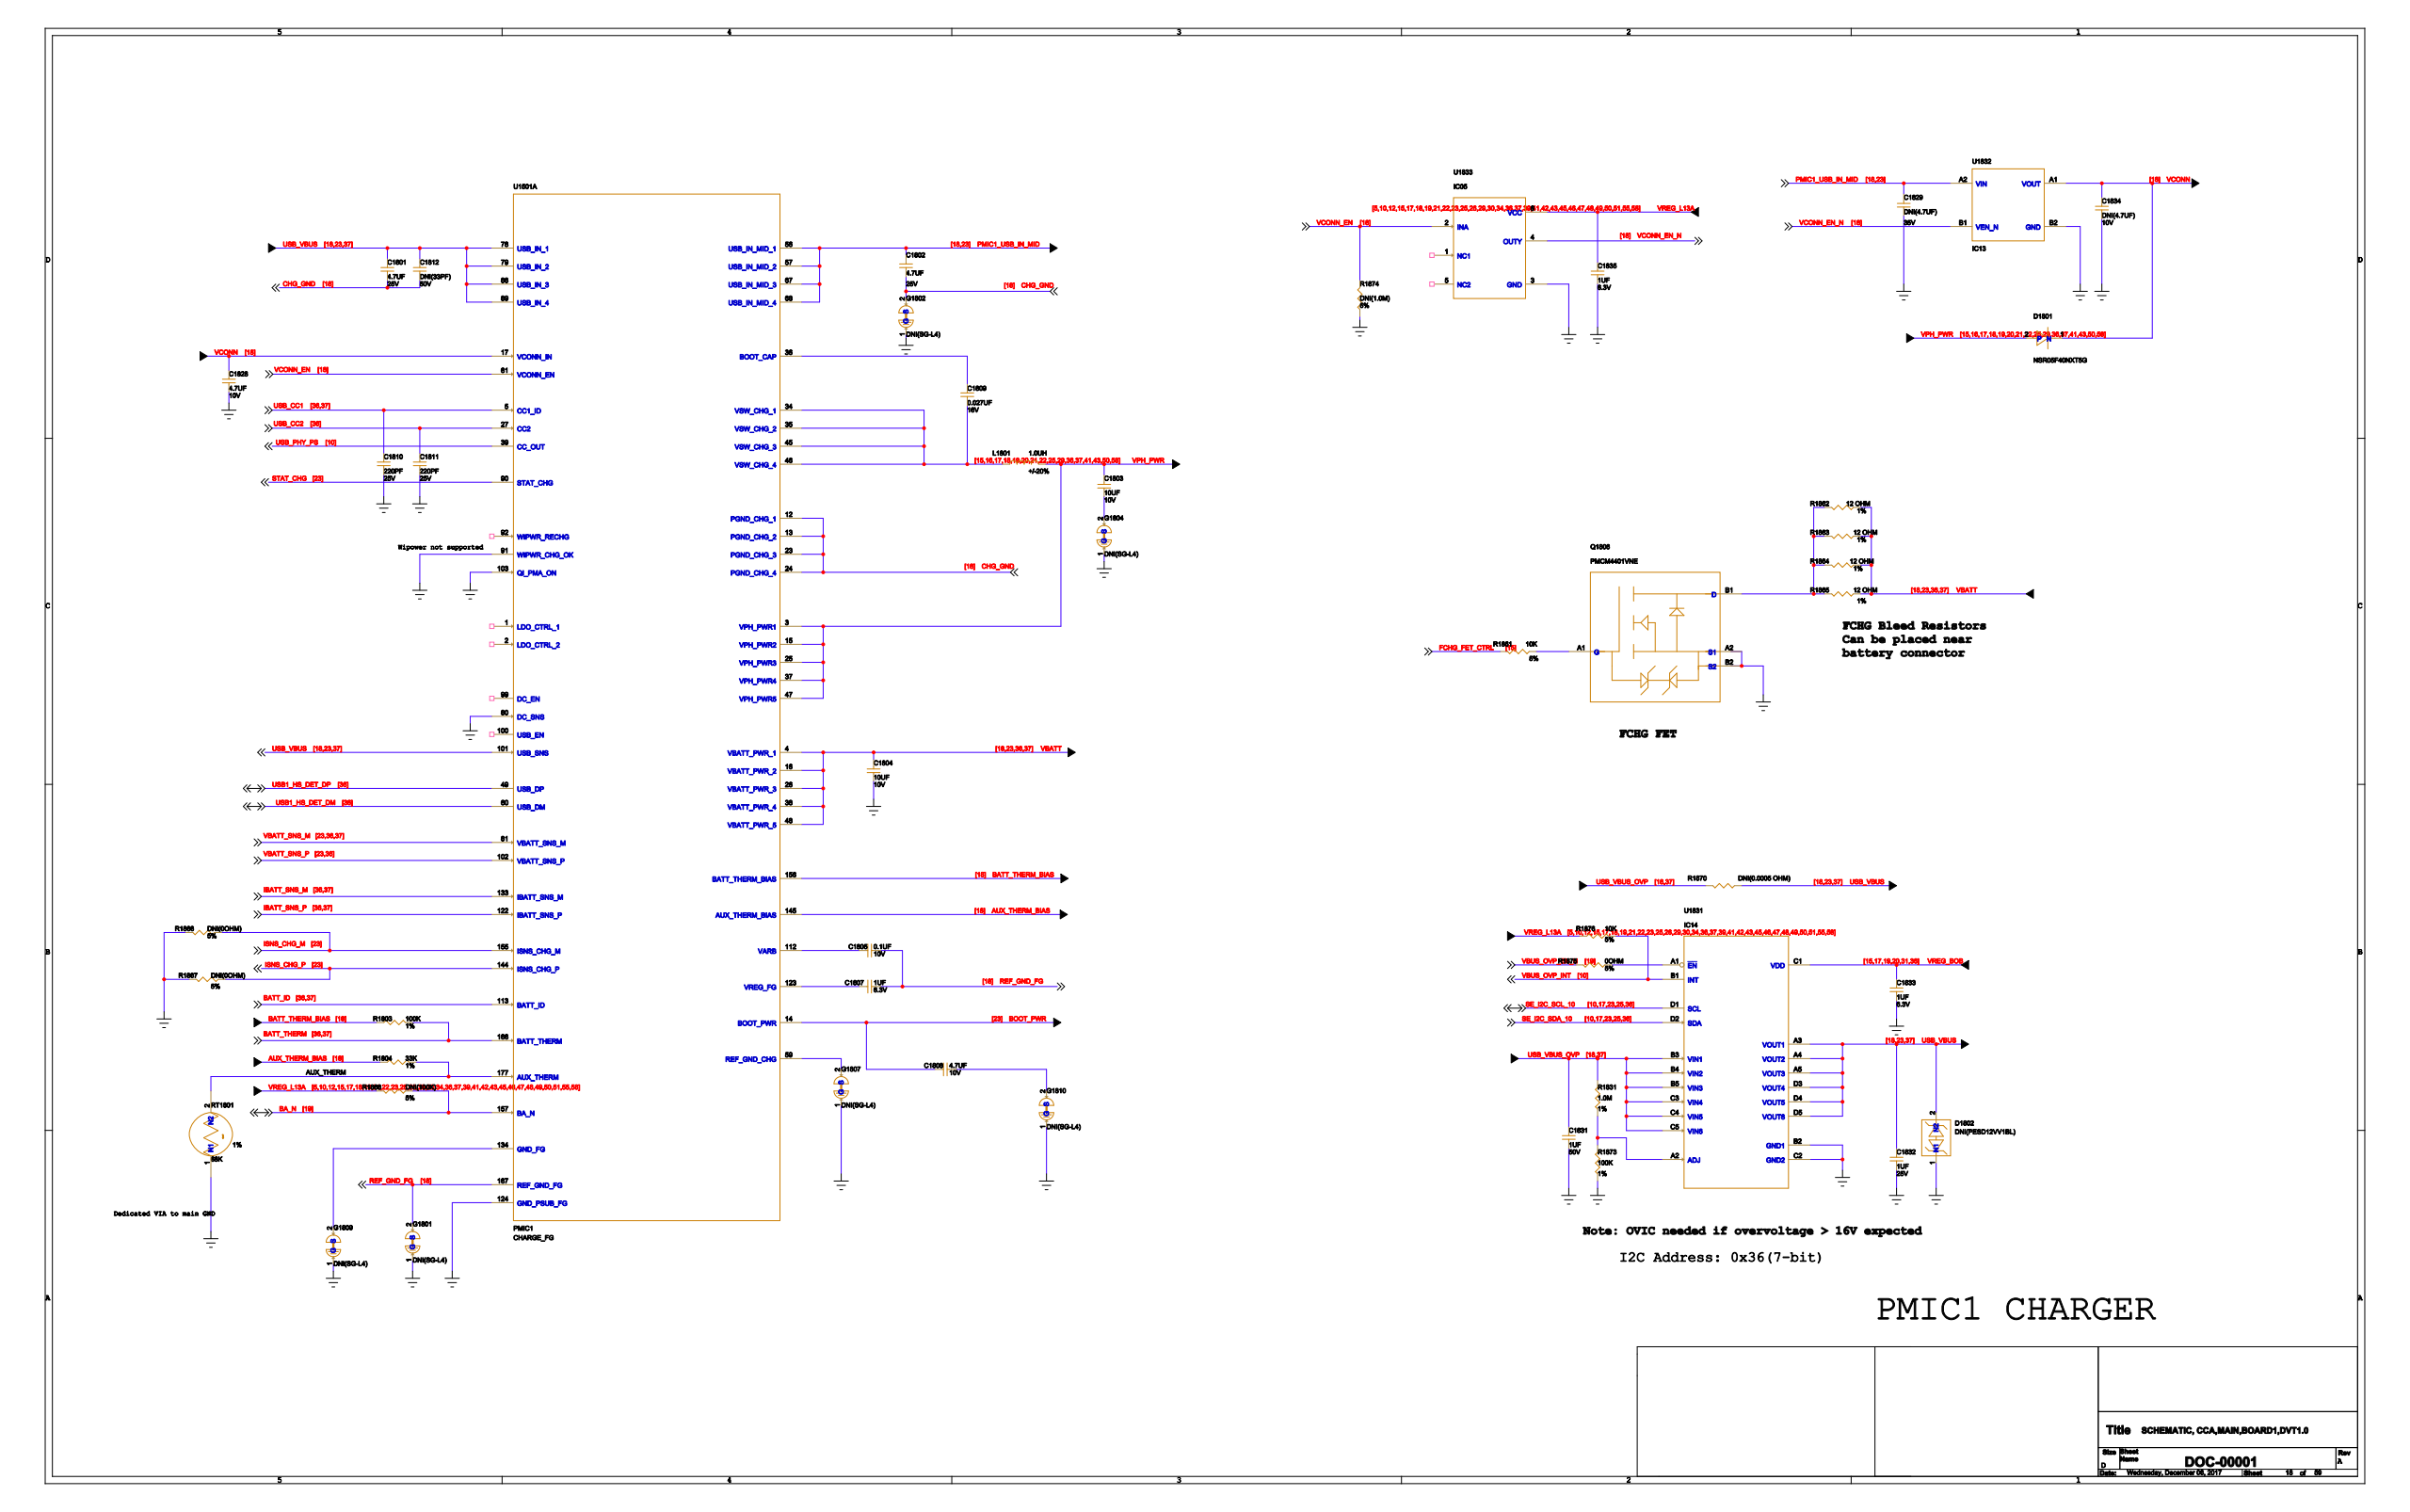Circuit board | KiCad | 1657 parts | 1365 nets | one sheet of the schematic
Parts on this sheet (reference | value | footprint):
C1801
C1802
C1803
C1804
C1805
C1807
C1808
C1809
C1810
C1811
C1812
C1828
C1829
C1831
C1832
C1833
C1834
C1835
D1801
D1802
G1801
G1802
G1804
G1807
G1809
G1810
L1801
Q1806
R1803
R1804
R1831
R1861
R1862
R1863
R1864
R1865
R1866
R1867
R1868
R1870
R1873
R1874
R1875
R1876
RT1801
U1501
U1831
U1832
U1833
Nets of these parts (net: part-pin ...):
GND: C1804-1 C1810-2 C1811-2 C1828-2 C1829-1 C1831-2 C1832-2 C1833-2 C1834-2 C1835-2 D1802-1 G1801-1 G1802-1 G1804-1 G1807-1 G1809-1 G1810-1 Q1806-A2 Q1806-B2 R1866-1 R1867-1 R1873-1 R1874-2 RT1801-1 U1831-B2 U1831-C2 U1832-B2 U1833-3 U1501-80 U1501-91 U1501-103 U1501-124
VREG_L13A: C1835-1 R1868-1 R1876-1 U1833-6
VPH_PWR: C1803-2 D1801-2 L1801-2 U1501-3 U1501-6 U1501-15 U1501-20 U1501-25 U1501-37 U1501-42 U1501-47 U1501-55
VBATT_SNS_P: U1501-102
IC1_USB_IN_MID: C1802-1 C1829-2 U1832-A2 U1501-56 U1501-57 U1501-67 U1501-68
BATT_THERM: R1803-1 U1501-166
AUX_THERM: R1804-1 RT1801-2 U1501-177
BOOT_PWR: C1808-1 U1501-14
STAT_CHG: U1501-90
USB_VBUS_OVP: C1831-1 R1831-2 R1870-1 U1831-B3 U1831-B4 U1831-B5 U1831-C3 U1831-C4 U1831-C5
USB1_HS_DET_DP: U1501-49
N22068067: R1875-1 U1831-A1
N21814736: R1831-1 R1873-2 U1831-A2
USB_VBUS: C1801-1 C1812-1 C1832-1 D1802-2 R1870-2 U1831-A3 U1831-A4 U1831-A5 U1831-D3 U1831-D4 U1831-D5 U1501-78 U1501-79 U1501-88 U1501-89 U1501-101
VBUS_OVP_INT: R1876-2 U1831-B1
VREG_BOB: C1833-1 U1831-C1
SE_I2C_SCL_10: U1831-D1
SE_I2C_SDA_10: U1831-D2
VBATT: C1804-2 R1862-2 R1863-2 R1864-2 R1865-2 U1501-4 U1501-16 U1501-26 U1501-38 U1501-48
N22312150: Q1806-B1 R1862-1 R1863-1 R1864-1 R1865-1
REF_GND_FG: C1805-2 C1807-2 G1801-2 U1501-167
IBATT_SNS_M: U1501-133
CHG_GND: C1801-2 C1802-2 C1812-2 G1802-2 U1501-12 U1501-13 U1501-23 U1501-24
FCHG_FET_CTRL: R1861-1
N22312183: Q1806-A1 R1861-2
USB_CC1: C1810-1 U1501-5
BATT_ID: U1501-113
VBATT_SNS_M: U1501-81
USB1_HS_DET_DM: U1501-60
ISNS_CHG_M: R1866-2 U1501-155
VBUS_OVP_EN_N: R1875-2
USB_PHY_PS: U1501-39
IBATT_SNS_P: U1501-122
N20089405: C1808-2 G1810-2
ISNS_CHG_P: R1867-2 U1501-144
N20088753: G1807-2 U1501-59
USB_CC2: C1811-1 U1501-27
N20089566: G1809-2 U1501-134
N20088715: C1803-1 G1804-2
ATT_THERM_BIAS: R1803-2 U1501-156
VCONN: C1828-1 C1834-1 D1801-1 U1832-A1 U1501-17
N20089435: C1807-1 U1501-123
NET_1366: U1833-1
VCONN_EN: R1874-1 U1833-2 U1501-61
VCONN_EN_N: U1832-B1 U1833-4
NET_1365: U1833-5
AUX_THERM_BIAS: R1804-2 U1501-145
N20089433: C1805-1 U1501-112
BA_N: R1868-2 U1501-157
N20088699: C1809-2 L1801-1 U1501-34 U1501-35 U1501-45 U1501-46
N20088693: C1809-1 U1501-36